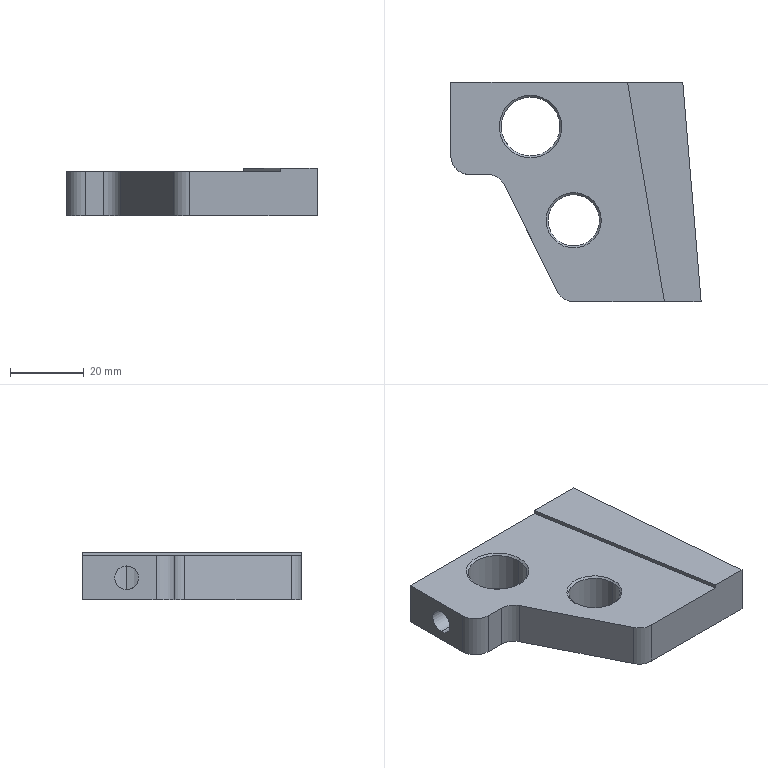Part | SolidWorks | features ICE 2, Chamfer 1, Extrusion 1 | 1 solid | 27 faces | box 68 x 59.543 x 13 mm | volume 33747 mm3 | plane 10 | cylinder 9 | cone 8 | commonest cylinder face diameters 10 x3 6.5 x2 14 x2 16 x2
STEP:
#1=CARTESIAN_POINT('',(13.645,13.,9.25));
#2=VERTEX_POINT('',#1);
#3=CARTESIAN_POINT('',(13.645,13.,2.75));
#4=VERTEX_POINT('',#3);
#5=CARTESIAN_POINT('',(13.645,13.,9.25));
#6=CARTESIAN_POINT('',(13.645,12.783,9.25));
#7=CARTESIAN_POINT('',(13.654,12.57,9.228));
#8=CARTESIAN_POINT('',(13.688,12.151,9.144));
#9=CARTESIAN_POINT('',(13.713,11.943,9.081));
#10=CARTESIAN_POINT('',(13.775,11.55,8.917));
#11=CARTESIAN_POINT('',(13.812,11.364,8.816));
#12=CARTESIAN_POINT('',(13.894,11.013,8.58));
#13=CARTESIAN_POINT('',(13.938,10.848,8.445));
#14=CARTESIAN_POINT('',(14.027,10.552,8.148));
#15=CARTESIAN_POINT('',(14.072,10.418,7.985));
#16=CARTESIAN_POINT('',(14.157,10.182,7.633));
#17=CARTESIAN_POINT('',(14.196,10.082,7.447));
#18=CARTESIAN_POINT('',(14.262,9.919,7.057));
#19=CARTESIAN_POINT('',(14.289,9.856,6.85));
#20=CARTESIAN_POINT('',(14.325,9.771,6.429));
#21=CARTESIAN_POINT('',(14.335,9.75,6.217));
#22=CARTESIAN_POINT('',(14.335,9.75,5.787));
#23=CARTESIAN_POINT('',(14.325,9.772,5.569));
#24=CARTESIAN_POINT('',(14.289,9.856,5.15));
#25=CARTESIAN_POINT('',(14.262,9.918,4.946));
#26=CARTESIAN_POINT('',(14.195,10.083,4.55));
#27=CARTESIAN_POINT('',(14.156,10.184,4.365));
#28=CARTESIAN_POINT('',(14.072,10.418,4.015));
#29=CARTESIAN_POINT('',(14.027,10.554,3.85));
#30=CARTESIAN_POINT('',(13.937,10.851,3.553));
#31=CARTESIAN_POINT('',(13.894,11.013,3.419));
#32=CARTESIAN_POINT('',(13.812,11.365,3.184));
#33=CARTESIAN_POINT('',(13.774,11.554,3.082));
#34=CARTESIAN_POINT('',(13.713,11.944,2.919));
#35=CARTESIAN_POINT('',(13.688,12.148,2.856));
#36=CARTESIAN_POINT('',(13.654,12.572,2.771));
#37=CARTESIAN_POINT('',(13.645,12.786,2.75));
#38=CARTESIAN_POINT('',(13.645,13.,2.75));
#39=B_SPLINE_CURVE_WITH_KNOTS('',3,(#5,#6,#7,#8,#9,#10,#11,#12,#13,#14,#15,#16,#17,#18,#19,#20,#21,#22,#23,#24,#25,#26,#27,#28,#29,#30,#31,#32,#33,#34,#35,#36,#37,#38),.UNSPECIFIED.,.F.,.F.,(4,2,2,2,2,2,2,2,2,2,2,2,2,2,2,2,4),(0.,0.0006421,0.001284,0.001926,0.002568,0.00321,0.003852,0.004495,0.005137,0.005779,0.006421,0.007063,0.007705,0.008347,0.008989,0.009631,0.01027),.UNSPECIFIED.);
#40=EDGE_CURVE('',#2,#4,#39,.T.);
#41=ORIENTED_EDGE('',*,*,#40,.T.);
#42=CARTESIAN_POINT('',(0.,13.,2.75));
#43=VERTEX_POINT('',#42);
#44=CARTESIAN_POINT('',(17.,13.,2.75));
#45=DIRECTION('',(-1.,0.,0.));
#46=VECTOR('',#45,1000.);
#47=LINE('',#44,#46);
#48=EDGE_CURVE('',#4,#43,#47,.T.);
#49=ORIENTED_EDGE('',*,*,#48,.T.);
#50=CARTESIAN_POINT('',(0.,13.,9.25));
#51=VERTEX_POINT('',#50);
#52=CARTESIAN_POINT('',(0.,13.,6.));
#53=DIRECTION('',(-1.,0.,0.));
#54=DIRECTION('',(0.,0.,1.));
#55=AXIS2_PLACEMENT_3D('',#52,#53,#54);
#56=CIRCLE('',#55,3.25);
#57=EDGE_CURVE('',#43,#51,#56,.T.);
#58=ORIENTED_EDGE('',*,*,#57,.T.);
#59=CARTESIAN_POINT('',(17.,13.,9.25));
#60=DIRECTION('',(-1.,0.,0.));
#61=VECTOR('',#60,1000.);
#62=LINE('',#59,#61);
#63=EDGE_CURVE('',#2,#51,#62,.T.);
#64=ORIENTED_EDGE('',*,*,#63,.F.);
#65=EDGE_LOOP('',(#41,#49,#58,#64));
#66=FACE_OUTER_BOUND('',#65,.T.);
#67=CARTESIAN_POINT('',(17.,13.,6.));
#68=DIRECTION('',(-1.,0.,0.));
#69=DIRECTION('',(0.,0.,1.));
#70=AXIS2_PLACEMENT_3D('',#67,#68,#69);
#71=CYLINDRICAL_SURFACE('',#70,3.25);
#72=ADVANCED_FACE('',(#66),#71,.F.);
#73=CARTESIAN_POINT('',(40.385,-12.47,0.5));
#74=VERTEX_POINT('',#73);
#75=CARTESIAN_POINT('',(26.385,-12.47,0.5));
#76=VERTEX_POINT('',#75);
#77=CARTESIAN_POINT('',(33.385,-12.47,0.5));
#78=DIRECTION('',(0.,0.,-1.));
#79=DIRECTION('',(1.,0.,0.));
#80=AXIS2_PLACEMENT_3D('',#77,#78,#79);
#81=CIRCLE('',#80,7.);
#82=EDGE_CURVE('',#74,#76,#81,.T.);
#83=ORIENTED_EDGE('',*,*,#82,.F.);
#84=CARTESIAN_POINT('',(40.885,-12.47,0.));
#85=VERTEX_POINT('',#84);
#86=CARTESIAN_POINT('',(40.885,-12.47,0.));
#87=DIRECTION('',(0.7071,0.,-0.7071));
#88=VECTOR('',#87,1000.);
#89=LINE('',#86,#88);
#90=EDGE_CURVE('',#74,#85,#89,.T.);
#91=ORIENTED_EDGE('',*,*,#90,.T.);
#92=CARTESIAN_POINT('',(25.885,-12.47,0.));
#93=VERTEX_POINT('',#92);
#94=CARTESIAN_POINT('',(33.385,-12.47,0.));
#95=DIRECTION('',(0.,0.,1.));
#96=DIRECTION('',(1.,0.,0.));
#97=AXIS2_PLACEMENT_3D('',#94,#95,#96);
#98=CIRCLE('',#97,7.5);
#99=EDGE_CURVE('',#93,#85,#98,.T.);
#100=ORIENTED_EDGE('',*,*,#99,.F.);
#101=CARTESIAN_POINT('',(25.885,-12.47,0.));
#102=DIRECTION('',(-0.7071,0.,-0.7071));
#103=VECTOR('',#102,1000.);
#104=LINE('',#101,#103);
#105=EDGE_CURVE('',#76,#93,#104,.T.);
#106=ORIENTED_EDGE('',*,*,#105,.F.);
#107=EDGE_LOOP('',(#83,#91,#100,#106));
#108=FACE_OUTER_BOUND('',#107,.T.);
#109=CARTESIAN_POINT('',(33.385,-12.47,0.));
#110=DIRECTION('',(0.,0.,-1.));
#111=DIRECTION('',(-1.,0.,0.));
#112=AXIS2_PLACEMENT_3D('',#109,#110,#111);
#113=CONICAL_SURFACE('',#112,7.5,0.7854);
#114=ADVANCED_FACE('',(#108),#113,.F.);
#115=CARTESIAN_POINT('',(29.645,13.,0.5));
#116=VERTEX_POINT('',#115);
#117=CARTESIAN_POINT('',(13.645,13.,0.5));
#118=VERTEX_POINT('',#117);
#119=CARTESIAN_POINT('',(21.645,13.,0.5));
#120=DIRECTION('',(0.,0.,-1.));
#121=DIRECTION('',(1.,0.,0.));
#122=AXIS2_PLACEMENT_3D('',#119,#120,#121);
#123=CIRCLE('',#122,8.);
#124=EDGE_CURVE('',#116,#118,#123,.T.);
#125=ORIENTED_EDGE('',*,*,#124,.F.);
#126=CARTESIAN_POINT('',(30.145,13.,0.));
#127=VERTEX_POINT('',#126);
#128=CARTESIAN_POINT('',(30.145,13.,0.));
#129=DIRECTION('',(0.7071,0.,-0.7071));
#130=VECTOR('',#129,1000.);
#131=LINE('',#128,#130);
#132=EDGE_CURVE('',#116,#127,#131,.T.);
#133=ORIENTED_EDGE('',*,*,#132,.T.);
#134=CARTESIAN_POINT('',(13.145,13.,0.));
#135=VERTEX_POINT('',#134);
#136=CARTESIAN_POINT('',(21.645,13.,0.));
#137=DIRECTION('',(0.,0.,1.));
#138=DIRECTION('',(1.,0.,0.));
#139=AXIS2_PLACEMENT_3D('',#136,#137,#138);
#140=CIRCLE('',#139,8.5);
#141=EDGE_CURVE('',#135,#127,#140,.T.);
#142=ORIENTED_EDGE('',*,*,#141,.F.);
#143=CARTESIAN_POINT('',(13.145,13.,0.));
#144=DIRECTION('',(-0.7071,0.,-0.7071));
#145=VECTOR('',#144,1000.);
#146=LINE('',#143,#145);
#147=EDGE_CURVE('',#118,#135,#146,.T.);
#148=ORIENTED_EDGE('',*,*,#147,.F.);
#149=EDGE_LOOP('',(#125,#133,#142,#148));
#150=FACE_OUTER_BOUND('',#149,.T.);
#151=CARTESIAN_POINT('',(21.645,13.,0.));
#152=DIRECTION('',(0.,0.,-1.));
#153=DIRECTION('',(-1.,0.,0.));
#154=AXIS2_PLACEMENT_3D('',#151,#152,#153);
#155=CONICAL_SURFACE('',#154,8.5,0.7854);
#156=ADVANCED_FACE('',(#150),#155,.F.);
#157=CARTESIAN_POINT('',(13.645,13.,11.5));
#158=VERTEX_POINT('',#157);
#159=CARTESIAN_POINT('',(29.645,13.,11.5));
#160=VERTEX_POINT('',#159);
#161=CARTESIAN_POINT('',(21.645,13.,11.5));
#162=DIRECTION('',(0.,0.,1.));
#163=DIRECTION('',(1.,0.,0.));
#164=AXIS2_PLACEMENT_3D('',#161,#162,#163);
#165=CIRCLE('',#164,8.);
#166=EDGE_CURVE('',#158,#160,#165,.T.);
#167=ORIENTED_EDGE('',*,*,#166,.F.);
#168=CARTESIAN_POINT('',(13.145,13.,12.));
#169=VERTEX_POINT('',#168);
#170=CARTESIAN_POINT('',(13.645,13.,11.5));
#171=DIRECTION('',(-0.7071,0.,0.7071));
#172=VECTOR('',#171,1000.);
#173=LINE('',#170,#172);
#174=EDGE_CURVE('',#158,#169,#173,.T.);
#175=ORIENTED_EDGE('',*,*,#174,.T.);
#176=CARTESIAN_POINT('',(30.145,13.,12.));
#177=VERTEX_POINT('',#176);
#178=CARTESIAN_POINT('',(21.645,13.,12.));
#179=DIRECTION('',(0.,0.,-1.));
#180=DIRECTION('',(1.,0.,0.));
#181=AXIS2_PLACEMENT_3D('',#178,#179,#180);
#182=CIRCLE('',#181,8.5);
#183=EDGE_CURVE('',#177,#169,#182,.T.);
#184=ORIENTED_EDGE('',*,*,#183,.F.);
#185=CARTESIAN_POINT('',(29.645,13.,11.5));
#186=DIRECTION('',(0.7071,0.,0.7071));
#187=VECTOR('',#186,1000.);
#188=LINE('',#185,#187);
#189=EDGE_CURVE('',#160,#177,#188,.T.);
#190=ORIENTED_EDGE('',*,*,#189,.F.);
#191=EDGE_LOOP('',(#167,#175,#184,#190));
#192=FACE_OUTER_BOUND('',#191,.T.);
#193=CARTESIAN_POINT('',(21.645,13.,11.5));
#194=DIRECTION('',(0.,0.,1.));
#195=DIRECTION('',(1.,0.,0.));
#196=AXIS2_PLACEMENT_3D('',#193,#194,#195);
#197=CONICAL_SURFACE('',#196,8.,0.7854);
#198=ADVANCED_FACE('',(#192),#197,.F.);
#199=CARTESIAN_POINT('',(26.385,-12.47,11.5));
#200=VERTEX_POINT('',#199);
#201=CARTESIAN_POINT('',(40.385,-12.47,11.5));
#202=VERTEX_POINT('',#201);
#203=CARTESIAN_POINT('',(33.385,-12.47,11.5));
#204=DIRECTION('',(0.,0.,1.));
#205=DIRECTION('',(1.,0.,0.));
#206=AXIS2_PLACEMENT_3D('',#203,#204,#205);
#207=CIRCLE('',#206,7.);
#208=EDGE_CURVE('',#200,#202,#207,.T.);
#209=ORIENTED_EDGE('',*,*,#208,.F.);
#210=CARTESIAN_POINT('',(25.885,-12.47,12.));
#211=VERTEX_POINT('',#210);
#212=CARTESIAN_POINT('',(26.385,-12.47,11.5));
#213=DIRECTION('',(-0.7071,0.,0.7071));
#214=VECTOR('',#213,1000.);
#215=LINE('',#212,#214);
#216=EDGE_CURVE('',#200,#211,#215,.T.);
#217=ORIENTED_EDGE('',*,*,#216,.T.);
#218=CARTESIAN_POINT('',(40.885,-12.47,12.));
#219=VERTEX_POINT('',#218);
#220=CARTESIAN_POINT('',(33.385,-12.47,12.));
#221=DIRECTION('',(0.,0.,-1.));
#222=DIRECTION('',(1.,0.,0.));
#223=AXIS2_PLACEMENT_3D('',#220,#221,#222);
#224=CIRCLE('',#223,7.5);
#225=EDGE_CURVE('',#219,#211,#224,.T.);
#226=ORIENTED_EDGE('',*,*,#225,.F.);
#227=CARTESIAN_POINT('',(40.385,-12.47,11.5));
#228=DIRECTION('',(0.7071,0.,0.7071));
#229=VECTOR('',#228,1000.);
#230=LINE('',#227,#229);
#231=EDGE_CURVE('',#202,#219,#230,.T.);
#232=ORIENTED_EDGE('',*,*,#231,.F.);
#233=EDGE_LOOP('',(#209,#217,#226,#232));
#234=FACE_OUTER_BOUND('',#233,.T.);
#235=CARTESIAN_POINT('',(33.385,-12.47,11.5));
#236=DIRECTION('',(0.,0.,1.));
#237=DIRECTION('',(1.,0.,0.));
#238=AXIS2_PLACEMENT_3D('',#235,#236,#237);
#239=CONICAL_SURFACE('',#238,7.,0.7854);
#240=ADVANCED_FACE('',(#234),#239,.F.);
#241=ORIENTED_EDGE('',*,*,#208,.T.);
#242=CARTESIAN_POINT('',(40.385,-12.47,13.));
#243=DIRECTION('',(0.,0.,-1.));
#244=VECTOR('',#243,1000.);
#245=LINE('',#242,#244);
#246=EDGE_CURVE('',#202,#74,#245,.T.);
#247=ORIENTED_EDGE('',*,*,#246,.T.);
#248=ORIENTED_EDGE('',*,*,#82,.T.);
#249=CARTESIAN_POINT('',(26.385,-12.47,13.));
#250=DIRECTION('',(0.,0.,-1.));
#251=VECTOR('',#250,1000.);
#252=LINE('',#249,#251);
#253=EDGE_CURVE('',#200,#76,#252,.T.);
#254=ORIENTED_EDGE('',*,*,#253,.F.);
#255=EDGE_LOOP('',(#241,#247,#248,#254));
#256=FACE_OUTER_BOUND('',#255,.T.);
#257=CARTESIAN_POINT('',(33.385,-12.47,13.));
#258=DIRECTION('',(0.,0.,-1.));
#259=DIRECTION('',(-1.,0.,0.));
#260=AXIS2_PLACEMENT_3D('',#257,#258,#259);
#261=CYLINDRICAL_SURFACE('',#260,7.);
#262=ADVANCED_FACE('',(#256),#261,.F.);
#263=ORIENTED_EDGE('',*,*,#166,.T.);
#264=CARTESIAN_POINT('',(29.645,13.,13.));
#265=DIRECTION('',(0.,0.,-1.));
#266=VECTOR('',#265,1000.);
#267=LINE('',#264,#266);
#268=EDGE_CURVE('',#160,#116,#267,.T.);
#269=ORIENTED_EDGE('',*,*,#268,.T.);
#270=ORIENTED_EDGE('',*,*,#124,.T.);
#271=CARTESIAN_POINT('',(13.645,13.,13.));
#272=DIRECTION('',(0.,0.,-1.));
#273=VECTOR('',#272,1000.);
#274=LINE('',#271,#273);
#275=EDGE_CURVE('',#4,#118,#274,.T.);
#276=ORIENTED_EDGE('',*,*,#275,.F.);
#277=ORIENTED_EDGE('',*,*,#40,.F.);
#278=CARTESIAN_POINT('',(13.645,13.,13.));
#279=DIRECTION('',(0.,0.,-1.));
#280=VECTOR('',#279,1000.);
#281=LINE('',#278,#280);
#282=EDGE_CURVE('',#158,#2,#281,.T.);
#283=ORIENTED_EDGE('',*,*,#282,.F.);
#284=EDGE_LOOP('',(#263,#269,#270,#276,#277,#283));
#285=FACE_OUTER_BOUND('',#284,.T.);
#286=CARTESIAN_POINT('',(21.645,13.,13.));
#287=DIRECTION('',(0.,0.,-1.));
#288=DIRECTION('',(-1.,0.,0.));
#289=AXIS2_PLACEMENT_3D('',#286,#287,#288);
#290=CYLINDRICAL_SURFACE('',#289,8.);
#291=ADVANCED_FACE('',(#285),#290,.F.);
#292=CARTESIAN_POINT('',(0.,13.,6.));
#293=DIRECTION('',(-1.,0.,0.));
#294=DIRECTION('',(0.,0.,1.));
#295=AXIS2_PLACEMENT_3D('',#292,#293,#294);
#296=CIRCLE('',#295,3.25);
#297=EDGE_CURVE('',#51,#43,#296,.T.);
#298=ORIENTED_EDGE('',*,*,#297,.F.);
#299=ORIENTED_EDGE('',*,*,#57,.F.);
#300=EDGE_LOOP('',(#298,#299));
#301=FACE_BOUND('',#300,.T.);
#302=CARTESIAN_POINT('',(0.,25.,12.));
#303=VERTEX_POINT('',#302);
#304=CARTESIAN_POINT('',(0.,5.,12.));
#305=VERTEX_POINT('',#304);
#306=CARTESIAN_POINT('',(0.,25.,12.));
#307=DIRECTION('',(0.,-1.,0.));
#308=VECTOR('',#307,1000.);
#309=LINE('',#306,#308);
#310=EDGE_CURVE('',#303,#305,#309,.T.);
#311=ORIENTED_EDGE('',*,*,#310,.F.);
#312=CARTESIAN_POINT('',(0.,25.,0.));
#313=VERTEX_POINT('',#312);
#314=CARTESIAN_POINT('',(0.,25.,13.));
#315=DIRECTION('',(0.,0.,-1.));
#316=VECTOR('',#315,1000.);
#317=LINE('',#314,#316);
#318=EDGE_CURVE('',#303,#313,#317,.T.);
#319=ORIENTED_EDGE('',*,*,#318,.T.);
#320=CARTESIAN_POINT('',(0.,5.,0.));
#321=VERTEX_POINT('',#320);
#322=CARTESIAN_POINT('',(0.,5.,0.));
#323=DIRECTION('',(0.,-1.,0.));
#324=VECTOR('',#323,1000.);
#325=LINE('',#322,#324);
#326=EDGE_CURVE('',#313,#321,#325,.T.);
#327=ORIENTED_EDGE('',*,*,#326,.T.);
#328=CARTESIAN_POINT('',(0.,5.,13.));
#329=DIRECTION('',(0.,0.,-1.));
#330=VECTOR('',#329,1000.);
#331=LINE('',#328,#330);
#332=EDGE_CURVE('',#305,#321,#331,.T.);
#333=ORIENTED_EDGE('',*,*,#332,.F.);
#334=EDGE_LOOP('',(#311,#319,#327,#333));
#335=FACE_OUTER_BOUND('',#334,.T.);
#336=CARTESIAN_POINT('',(0.,5.,13.));
#337=DIRECTION('',(1.,0.,0.));
#338=DIRECTION('',(0.,0.,-1.));
#339=AXIS2_PLACEMENT_3D('',#336,#337,#338);
#340=PLANE('',#339);
#341=ADVANCED_FACE('',(#301,#335),#340,.F.);
#342=CARTESIAN_POINT('',(5.,0.,12.));
#343=VERTEX_POINT('',#342);
#344=CARTESIAN_POINT('',(5.,5.,12.));
#345=DIRECTION('',(0.,0.,1.));
#346=DIRECTION('',(1.,0.,0.));
#347=AXIS2_PLACEMENT_3D('',#344,#345,#346);
#348=CIRCLE('',#347,5.);
#349=EDGE_CURVE('',#305,#343,#348,.T.);
#350=ORIENTED_EDGE('',*,*,#349,.F.);
#351=ORIENTED_EDGE('',*,*,#332,.T.);
#352=CARTESIAN_POINT('',(5.,0.,0.));
#353=VERTEX_POINT('',#352);
#354=CARTESIAN_POINT('',(5.,5.,0.));
#355=DIRECTION('',(0.,0.,1.));
#356=DIRECTION('',(-1.,0.,0.));
#357=AXIS2_PLACEMENT_3D('',#354,#355,#356);
#358=CIRCLE('',#357,5.);
#359=EDGE_CURVE('',#321,#353,#358,.T.);
#360=ORIENTED_EDGE('',*,*,#359,.T.);
#361=CARTESIAN_POINT('',(5.,0.,13.));
#362=DIRECTION('',(0.,0.,-1.));
#363=VECTOR('',#362,1000.);
#364=LINE('',#361,#363);
#365=EDGE_CURVE('',#343,#353,#364,.T.);
#366=ORIENTED_EDGE('',*,*,#365,.F.);
#367=EDGE_LOOP('',(#350,#351,#360,#366));
#368=FACE_OUTER_BOUND('',#367,.T.);
#369=CARTESIAN_POINT('',(5.,5.,13.));
#370=DIRECTION('',(0.,0.,-1.));
#371=DIRECTION('',(-1.,0.,0.));
#372=AXIS2_PLACEMENT_3D('',#369,#370,#371);
#373=CYLINDRICAL_SURFACE('',#372,5.);
#374=ADVANCED_FACE('',(#368),#373,.T.);
#375=CARTESIAN_POINT('',(9.997,0.,12.));
#376=VERTEX_POINT('',#375);
#377=CARTESIAN_POINT('',(5.,0.,12.));
#378=DIRECTION('',(1.,0.,0.));
#379=VECTOR('',#378,1000.);
#380=LINE('',#377,#379);
#381=EDGE_CURVE('',#343,#376,#380,.T.);
#382=ORIENTED_EDGE('',*,*,#381,.F.);
#383=ORIENTED_EDGE('',*,*,#365,.T.);
#384=CARTESIAN_POINT('',(9.997,0.,0.));
#385=VERTEX_POINT('',#384);
#386=CARTESIAN_POINT('',(9.997,0.,0.));
#387=DIRECTION('',(1.,0.,0.));
#388=VECTOR('',#387,1000.);
#389=LINE('',#386,#388);
#390=EDGE_CURVE('',#353,#385,#389,.T.);
#391=ORIENTED_EDGE('',*,*,#390,.T.);
#392=CARTESIAN_POINT('',(9.997,0.,13.));
#393=DIRECTION('',(0.,0.,-1.));
#394=VECTOR('',#393,1000.);
#395=LINE('',#392,#394);
#396=EDGE_CURVE('',#376,#385,#395,.T.);
#397=ORIENTED_EDGE('',*,*,#396,.F.);
#398=EDGE_LOOP('',(#382,#383,#391,#397));
#399=FACE_OUTER_BOUND('',#398,.T.);
#400=CARTESIAN_POINT('',(9.997,0.,13.));
#401=DIRECTION('',(0.,1.,0.));
#402=DIRECTION('',(0.,0.,1.));
#403=AXIS2_PLACEMENT_3D('',#400,#401,#402);
#404=PLANE('',#403);
#405=ADVANCED_FACE('',(#399),#404,.F.);
#406=CARTESIAN_POINT('',(14.473,-2.772,12.));
#407=VERTEX_POINT('',#406);
#408=CARTESIAN_POINT('',(9.997,-5.,12.));
#409=DIRECTION('',(0.,0.,-1.));
#410=DIRECTION('',(1.,0.,0.));
#411=AXIS2_PLACEMENT_3D('',#408,#409,#410);
#412=CIRCLE('',#411,5.);
#413=EDGE_CURVE('',#376,#407,#412,.T.);
#414=ORIENTED_EDGE('',*,*,#413,.F.);
#415=ORIENTED_EDGE('',*,*,#396,.T.);
#416=CARTESIAN_POINT('',(14.473,-2.772,0.));
#417=VERTEX_POINT('',#416);
#418=CARTESIAN_POINT('',(9.997,-5.,0.));
#419=DIRECTION('',(0.,0.,-1.));
#420=DIRECTION('',(-1.,0.,0.));
#421=AXIS2_PLACEMENT_3D('',#418,#419,#420);
#422=CIRCLE('',#421,5.);
#423=EDGE_CURVE('',#385,#417,#422,.T.);
#424=ORIENTED_EDGE('',*,*,#423,.T.);
#425=CARTESIAN_POINT('',(14.473,-2.772,13.));
#426=DIRECTION('',(0.,0.,-1.));
#427=VECTOR('',#426,1000.);
#428=LINE('',#425,#427);
#429=EDGE_CURVE('',#407,#417,#428,.T.);
#430=ORIENTED_EDGE('',*,*,#429,.F.);
#431=EDGE_LOOP('',(#414,#415,#424,#430));
#432=FACE_OUTER_BOUND('',#431,.T.);
#433=CARTESIAN_POINT('',(9.997,-5.,13.));
#434=DIRECTION('',(0.,0.,-1.));
#435=DIRECTION('',(-1.,0.,0.));
#436=AXIS2_PLACEMENT_3D('',#433,#434,#435);
#437=CYLINDRICAL_SURFACE('',#436,5.);
#438=ADVANCED_FACE('',(#432),#437,.F.);
#439=CARTESIAN_POINT('',(28.909,-31.772,12.));
#440=VERTEX_POINT('',#439);
#441=CARTESIAN_POINT('',(14.473,-2.772,12.));
#442=DIRECTION('',(0.4456,-0.8952,0.));
#443=VECTOR('',#442,1000.);
#444=LINE('',#441,#443);
#445=EDGE_CURVE('',#407,#440,#444,.T.);
#446=ORIENTED_EDGE('',*,*,#445,.F.);
#447=ORIENTED_EDGE('',*,*,#429,.T.);
#448=CARTESIAN_POINT('',(28.909,-31.772,0.));
#449=VERTEX_POINT('',#448);
#450=CARTESIAN_POINT('',(28.909,-31.772,0.));
#451=DIRECTION('',(0.4456,-0.8952,0.));
#452=VECTOR('',#451,1000.);
#453=LINE('',#450,#452);
#454=EDGE_CURVE('',#417,#449,#453,.T.);
#455=ORIENTED_EDGE('',*,*,#454,.T.);
#456=CARTESIAN_POINT('',(28.909,-31.772,13.));
#457=DIRECTION('',(0.,0.,-1.));
#458=VECTOR('',#457,1000.);
#459=LINE('',#456,#458);
#460=EDGE_CURVE('',#440,#449,#459,.T.);
#461=ORIENTED_EDGE('',*,*,#460,.F.);
#462=EDGE_LOOP('',(#446,#447,#455,#461));
#463=FACE_OUTER_BOUND('',#462,.T.);
#464=CARTESIAN_POINT('',(28.909,-31.772,13.));
#465=DIRECTION('',(0.8952,0.4456,0.));
#466=DIRECTION('',(-0.4456,0.8952,0.));
#467=AXIS2_PLACEMENT_3D('',#464,#465,#466);
#468=PLANE('',#467);
#469=ADVANCED_FACE('',(#463),#468,.F.);
#470=CARTESIAN_POINT('',(33.385,-34.543,12.));
#471=VERTEX_POINT('',#470);
#472=CARTESIAN_POINT('',(33.385,-29.543,12.));
#473=DIRECTION('',(0.,0.,1.));
#474=DIRECTION('',(1.,0.,0.));
#475=AXIS2_PLACEMENT_3D('',#472,#473,#474);
#476=CIRCLE('',#475,5.);
#477=EDGE_CURVE('',#440,#471,#476,.T.);
#478=ORIENTED_EDGE('',*,*,#477,.F.);
#479=ORIENTED_EDGE('',*,*,#460,.T.);
#480=CARTESIAN_POINT('',(33.385,-34.543,0.));
#481=VERTEX_POINT('',#480);
#482=CARTESIAN_POINT('',(33.385,-29.543,0.));
#483=DIRECTION('',(0.,0.,1.));
#484=DIRECTION('',(1.,0.,0.));
#485=AXIS2_PLACEMENT_3D('',#482,#483,#484);
#486=CIRCLE('',#485,5.);
#487=EDGE_CURVE('',#449,#481,#486,.T.);
#488=ORIENTED_EDGE('',*,*,#487,.T.);
#489=CARTESIAN_POINT('',(33.385,-34.543,13.));
#490=DIRECTION('',(0.,0.,-1.));
#491=VECTOR('',#490,1000.);
#492=LINE('',#489,#491);
#493=EDGE_CURVE('',#471,#481,#492,.T.);
#494=ORIENTED_EDGE('',*,*,#493,.F.);
#495=EDGE_LOOP('',(#478,#479,#488,#494));
#496=FACE_OUTER_BOUND('',#495,.T.);
#497=CARTESIAN_POINT('',(33.385,-29.543,13.));
#498=DIRECTION('',(0.,0.,-1.));
#499=DIRECTION('',(-1.,0.,0.));
#500=AXIS2_PLACEMENT_3D('',#497,#498,#499);
#501=CYLINDRICAL_SURFACE('',#500,5.);
#502=ADVANCED_FACE('',(#496),#501,.T.);
#503=ORIENTED_EDGE('',*,*,#268,.F.);
#504=CARTESIAN_POINT('',(21.645,13.,11.5));
#505=DIRECTION('',(0.,0.,1.));
#506=DIRECTION('',(1.,0.,0.));
#507=AXIS2_PLACEMENT_3D('',#504,#505,#506);
#508=CIRCLE('',#507,8.);
#509=EDGE_CURVE('',#160,#158,#508,.T.);
#510=ORIENTED_EDGE('',*,*,#509,.T.);
#511=ORIENTED_EDGE('',*,*,#282,.T.);
#512=CARTESIAN_POINT('',(13.645,13.,2.75));
#513=CARTESIAN_POINT('',(13.645,13.214,2.75));
#514=CARTESIAN_POINT('',(13.654,13.431,2.772));
#515=CARTESIAN_POINT('',(13.688,13.852,2.856));
#516=CARTESIAN_POINT('',(13.713,14.055,2.919));
#517=CARTESIAN_POINT('',(13.775,14.449,3.083));
#518=CARTESIAN_POINT('',(13.812,14.638,3.185));
#519=CARTESIAN_POINT('',(13.894,14.987,3.42));
#520=CARTESIAN_POINT('',(13.938,15.15,3.554));
#521=CARTESIAN_POINT('',(14.028,15.45,3.854));
#522=CARTESIAN_POINT('',(14.072,15.582,4.016));
#523=CARTESIAN_POINT('',(14.156,15.816,4.365));
#524=CARTESIAN_POINT('',(14.196,15.918,4.554));
#525=CARTESIAN_POINT('',(14.262,16.082,4.946));
#526=CARTESIAN_POINT('',(14.289,16.144,5.148));
#527=CARTESIAN_POINT('',(14.325,16.228,5.567));
#528=CARTESIAN_POINT('',(14.335,16.25,5.785));
#529=CARTESIAN_POINT('',(14.335,16.25,6.214));
#530=CARTESIAN_POINT('',(14.326,16.229,6.427));
#531=CARTESIAN_POINT('',(14.289,16.144,6.85));
#532=CARTESIAN_POINT('',(14.262,16.081,7.055));
#533=CARTESIAN_POINT('',(14.196,15.918,7.446));
#534=CARTESIAN_POINT('',(14.156,15.816,7.635));
#535=CARTESIAN_POINT('',(14.072,15.581,7.986));
#536=CARTESIAN_POINT('',(14.027,15.448,8.148));
#537=CARTESIAN_POINT('',(13.938,15.15,8.446));
#538=CARTESIAN_POINT('',(13.893,14.986,8.582));
#539=CARTESIAN_POINT('',(13.812,14.637,8.816));
#540=CARTESIAN_POINT('',(13.775,14.451,8.916));
#541=CARTESIAN_POINT('',(13.712,14.055,9.082));
#542=CARTESIAN_POINT('',(13.688,13.851,9.144));
#543=CARTESIAN_POINT('',(13.654,13.433,9.228));
#544=CARTESIAN_POINT('',(13.645,13.217,9.25));
#545=CARTESIAN_POINT('',(13.645,13.,9.25));
#546=B_SPLINE_CURVE_WITH_KNOTS('',3,(#512,#513,#514,#515,#516,#517,#518,#519,#520,#521,#522,#523,#524,#525,#526,#527,#528,#529,#530,#531,#532,#533,#534,#535,#536,#537,#538,#539,#540,#541,#542,#543,#544,#545),.UNSPECIFIED.,.F.,.F.,(4,2,2,2,2,2,2,2,2,2,2,2,2,2,2,2,4),(0.01027,0.01091,0.01156,0.0122,0.01284,0.01348,0.01412,0.01476,0.01541,0.01605,0.01669,0.01733,0.01797,0.01861,0.01926,0.0199,0.02054),.UNSPECIFIED.);
#547=EDGE_CURVE('',#4,#2,#546,.T.);
#548=ORIENTED_EDGE('',*,*,#547,.F.);
#549=ORIENTED_EDGE('',*,*,#275,.T.);
#550=CARTESIAN_POINT('',(21.645,13.,0.5));
#551=DIRECTION('',(0.,0.,-1.));
#552=DIRECTION('',(1.,0.,0.));
#553=AXIS2_PLACEMENT_3D('',#550,#551,#552);
#554=CIRCLE('',#553,8.);
#555=EDGE_CURVE('',#118,#116,#554,.T.);
#556=ORIENTED_EDGE('',*,*,#555,.T.);
#557=EDGE_LOOP('',(#503,#510,#511,#548,#549,#556));
#558=FACE_OUTER_BOUND('',#557,.T.);
#559=CARTESIAN_POINT('',(21.645,13.,13.));
#560=DIRECTION('',(0.,0.,-1.));
#561=DIRECTION('',(-1.,0.,0.));
#562=AXIS2_PLACEMENT_3D('',#559,#560,#561);
#563=CYLINDRICAL_SURFACE('',#562,8.);
#564=ADVANCED_FACE('',(#558),#563,.F.);
#565=ORIENTED_EDGE('',*,*,#246,.F.);
#566=CARTESIAN_POINT('',(33.385,-12.47,11.5));
#567=DIRECTION('',(0.,0.,1.));
#568=DIRECTION('',(1.,0.,0.));
#569=AXIS2_PLACEMENT_3D('',#566,#567,#568);
#570=CIRCLE('',#569,7.);
#571=EDGE_CURVE('',#202,#200,#570,.T.);
#572=ORIENTED_EDGE('',*,*,#571,.T.);
#573=ORIENTED_EDGE('',*,*,#253,.T.);
#574=CARTESIAN_POINT('',(33.385,-12.47,0.5));
#575=DIRECTION('',(0.,0.,-1.));
#576=DIRECTION('',(1.,0.,0.));
#577=AXIS2_PLACEMENT_3D('',#574,#575,#576);
#578=CIRCLE('',#577,7.);
#579=EDGE_CURVE('',#76,#74,#578,.T.);
#580=ORIENTED_EDGE('',*,*,#579,.T.);
#581=EDGE_LOOP('',(#565,#572,#573,#580));
#582=FACE_OUTER_BOUND('',#581,.T.);
#583=CARTESIAN_POINT('',(33.385,-12.47,13.));
#584=DIRECTION('',(0.,0.,-1.));
#585=DIRECTION('',(-1.,0.,0.));
#586=AXIS2_PLACEMENT_3D('',#583,#584,#585);
#587=CYLINDRICAL_SURFACE('',#586,7.);
#588=ADVANCED_FACE('',(#582),#587,.F.);
#589=CARTESIAN_POINT('',(58.,-34.543,13.));
#590=VERTEX_POINT('',#589);
#591=CARTESIAN_POINT('',(48.,25.,13.));
#592=VERTEX_POINT('',#591);
#593=CARTESIAN_POINT('',(48.,25.,13.));
#594=DIRECTION('',(-0.1656,0.9862,0.));
#595=VECTOR('',#594,1000.);
#596=LINE('',#593,#595);
#597=EDGE_CURVE('',#590,#592,#596,.T.);
#598=ORIENTED_EDGE('',*,*,#597,.F.);
#599=CARTESIAN_POINT('',(68.,-34.543,13.));
#600=VERTEX_POINT('',#599);
#601=CARTESIAN_POINT('',(68.,-34.543,13.));
#602=DIRECTION('',(1.,0.,0.));
#603=VECTOR('',#602,1000.);
#604=LINE('',#601,#603);
#605=EDGE_CURVE('',#590,#600,#604,.T.);
#606=ORIENTED_EDGE('',*,*,#605,.T.);
#607=CARTESIAN_POINT('',(63.,25.,13.));
#608=VERTEX_POINT('',#607);
#609=CARTESIAN_POINT('',(63.,25.,13.));
#610=DIRECTION('',(-0.08368,0.9965,0.));
#611=VECTOR('',#610,1000.);
#612=LINE('',#609,#611);
#613=EDGE_CURVE('',#600,#608,#612,.T.);
#614=ORIENTED_EDGE('',*,*,#613,.T.);
#615=CARTESIAN_POINT('',(0.,25.,13.));
#616=DIRECTION('',(-1.,0.,0.));
#617=VECTOR('',#616,1000.);
#618=LINE('',#615,#617);
#619=EDGE_CURVE('',#608,#592,#618,.T.);
#620=ORIENTED_EDGE('',*,*,#619,.T.);
#621=EDGE_LOOP('',(#598,#606,#614,#620));
#622=FACE_OUTER_BOUND('',#621,.T.);
#623=CARTESIAN_POINT('',(33.385,-29.543,13.));
#624=DIRECTION('',(0.,0.,1.));
#625=DIRECTION('',(1.,0.,0.));
#626=AXIS2_PLACEMENT_3D('',#623,#624,#625);
#627=PLANE('',#626);
#628=ADVANCED_FACE('',(#622),#627,.T.);
#629=ORIENTED_EDGE('',*,*,#141,.T.);
#630=CARTESIAN_POINT('',(21.645,13.,0.));
#631=DIRECTION('',(0.,0.,1.));
#632=DIRECTION('',(1.,0.,0.));
#633=AXIS2_PLACEMENT_3D('',#630,#631,#632);
#634=CIRCLE('',#633,8.5);
#635=EDGE_CURVE('',#127,#135,#634,.T.);
#636=ORIENTED_EDGE('',*,*,#635,.T.);
#637=EDGE_LOOP('',(#629,#636));
#638=FACE_BOUND('',#637,.T.);
#639=ORIENTED_EDGE('',*,*,#99,.T.);
#640=CARTESIAN_POINT('',(33.385,-12.47,0.));
#641=DIRECTION('',(0.,0.,1.));
#642=DIRECTION('',(1.,0.,0.));
#643=AXIS2_PLACEMENT_3D('',#640,#641,#642);
#644=CIRCLE('',#643,7.5);
#645=EDGE_CURVE('',#85,#93,#644,.T.);
#646=ORIENTED_EDGE('',*,*,#645,.T.);
#647=EDGE_LOOP('',(#639,#646));
#648=FACE_BOUND('',#647,.T.);
#649=CARTESIAN_POINT('',(63.,25.,0.));
#650=VERTEX_POINT('',#649);
#651=CARTESIAN_POINT('',(0.,25.,0.));
#652=DIRECTION('',(-1.,0.,0.));
#653=VECTOR('',#652,1000.);
#654=LINE('',#651,#653);
#655=EDGE_CURVE('',#650,#313,#654,.T.);
#656=ORIENTED_EDGE('',*,*,#655,.F.);
#657=CARTESIAN_POINT('',(68.,-34.543,0.));
#658=VERTEX_POINT('',#657);
#659=CARTESIAN_POINT('',(63.,25.,0.));
#660=DIRECTION('',(-0.08368,0.9965,0.));
#661=VECTOR('',#660,1000.);
#662=LINE('',#659,#661);
#663=EDGE_CURVE('',#658,#650,#662,.T.);
#664=ORIENTED_EDGE('',*,*,#663,.F.);
#665=CARTESIAN_POINT('',(68.,-34.543,0.));
#666=DIRECTION('',(1.,0.,0.));
#667=VECTOR('',#666,1000.);
#668=LINE('',#665,#667);
#669=EDGE_CURVE('',#481,#658,#668,.T.);
#670=ORIENTED_EDGE('',*,*,#669,.F.);
#671=ORIENTED_EDGE('',*,*,#487,.F.);
#672=ORIENTED_EDGE('',*,*,#454,.F.);
#673=ORIENTED_EDGE('',*,*,#423,.F.);
#674=ORIENTED_EDGE('',*,*,#390,.F.);
#675=ORIENTED_EDGE('',*,*,#359,.F.);
#676=ORIENTED_EDGE('',*,*,#326,.F.);
#677=EDGE_LOOP('',(#656,#664,#670,#671,#672,#673,#674,#675,#676));
#678=FACE_OUTER_BOUND('',#677,.T.);
#679=CARTESIAN_POINT('',(33.385,-29.543,0.));
#680=DIRECTION('',(0.,0.,1.));
#681=DIRECTION('',(1.,0.,0.));
#682=AXIS2_PLACEMENT_3D('',#679,#680,#681);
#683=PLANE('',#682);
#684=ADVANCED_FACE('',(#638,#648,#678),#683,.F.);
#685=CARTESIAN_POINT('',(48.,25.,12.));
#686=VERTEX_POINT('',#685);
#687=CARTESIAN_POINT('',(48.,25.,12.));
#688=DIRECTION('',(-1.,0.,0.));
#689=VECTOR('',#688,1000.);
#690=LINE('',#687,#689);
#691=EDGE_CURVE('',#686,#303,#690,.T.);
#692=ORIENTED_EDGE('',*,*,#691,.F.);
#693=CARTESIAN_POINT('',(48.,25.,12.));
#694=DIRECTION('',(0.,0.,1.));
#695=VECTOR('',#694,1000.);
#696=LINE('',#693,#695);
#697=EDGE_CURVE('',#686,#592,#696,.T.);
#698=ORIENTED_EDGE('',*,*,#697,.T.);
#699=ORIENTED_EDGE('',*,*,#619,.F.);
#700=CARTESIAN_POINT('',(63.,25.,13.));
#701=DIRECTION('',(0.,0.,-1.));
#702=VECTOR('',#701,1000.);
#703=LINE('',#700,#702);
#704=EDGE_CURVE('',#608,#650,#703,.T.);
#705=ORIENTED_EDGE('',*,*,#704,.T.);
#706=ORIENTED_EDGE('',*,*,#655,.T.);
#707=ORIENTED_EDGE('',*,*,#318,.F.);
#708=EDGE_LOOP('',(#692,#698,#699,#705,#706,#707));
#709=FACE_OUTER_BOUND('',#708,.T.);
#710=CARTESIAN_POINT('',(0.,25.,13.));
#711=DIRECTION('',(0.,-1.,0.));
#712=DIRECTION('',(0.,0.,-1.));
#713=AXIS2_PLACEMENT_3D('',#710,#711,#712);
#714=PLANE('',#713);
#715=ADVANCED_FACE('',(#709),#714,.F.);
#716=ORIENTED_EDGE('',*,*,#605,.F.);
#717=CARTESIAN_POINT('',(58.,-34.543,12.));
#718=VERTEX_POINT('',#717);
#719=CARTESIAN_POINT('',(58.,-34.543,12.));
#720=DIRECTION('',(0.,0.,1.));
#721=VECTOR('',#720,1000.);
#722=LINE('',#719,#721);
#723=EDGE_CURVE('',#718,#590,#722,.T.);
#724=ORIENTED_EDGE('',*,*,#723,.F.);
#725=CARTESIAN_POINT('',(33.385,-34.543,12.));
#726=DIRECTION('',(1.,0.,0.));
#727=VECTOR('',#726,1000.);
#728=LINE('',#725,#727);
#729=EDGE_CURVE('',#471,#718,#728,.T.);
#730=ORIENTED_EDGE('',*,*,#729,.F.);
#731=ORIENTED_EDGE('',*,*,#493,.T.);
#732=ORIENTED_EDGE('',*,*,#669,.T.);
#733=CARTESIAN_POINT('',(68.,-34.543,13.));
#734=DIRECTION('',(0.,0.,-1.));
#735=VECTOR('',#734,1000.);
#736=LINE('',#733,#735);
#737=EDGE_CURVE('',#600,#658,#736,.T.);
#738=ORIENTED_EDGE('',*,*,#737,.F.);
#739=EDGE_LOOP('',(#716,#724,#730,#731,#732,#738));
#740=FACE_OUTER_BOUND('',#739,.T.);
#741=CARTESIAN_POINT('',(68.,-34.543,13.));
#742=DIRECTION('',(0.,1.,0.));
#743=DIRECTION('',(0.,0.,1.));
#744=AXIS2_PLACEMENT_3D('',#741,#742,#743);
#745=PLANE('',#744);
#746=ADVANCED_FACE('',(#740),#745,.F.);
#747=ORIENTED_EDGE('',*,*,#663,.T.);
#748=ORIENTED_EDGE('',*,*,#704,.F.);
#749=ORIENTED_EDGE('',*,*,#613,.F.);
#750=ORIENTED_EDGE('',*,*,#737,.T.);
#751=EDGE_LOOP('',(#747,#748,#749,#750));
#752=FACE_OUTER_BOUND('',#751,.T.);
#753=CARTESIAN_POINT('',(63.,25.,13.));
#754=DIRECTION('',(-0.9965,-0.08368,0.));
#755=DIRECTION('',(0.08368,-0.9965,0.));
#756=AXIS2_PLACEMENT_3D('',#753,#754,#755);
#757=PLANE('',#756);
#758=ADVANCED_FACE('',(#752),#757,.F.);
#759=ORIENTED_EDGE('',*,*,#597,.T.);
#760=ORIENTED_EDGE('',*,*,#697,.F.);
#761=CARTESIAN_POINT('',(48.,25.,12.));
#762=DIRECTION('',(-0.1656,0.9862,0.));
#763=VECTOR('',#762,1000.);
#764=LINE('',#761,#763);
#765=EDGE_CURVE('',#718,#686,#764,.T.);
#766=ORIENTED_EDGE('',*,*,#765,.F.);
#767=ORIENTED_EDGE('',*,*,#723,.T.);
#768=EDGE_LOOP('',(#759,#760,#766,#767));
#769=FACE_OUTER_BOUND('',#768,.T.);
#770=CARTESIAN_POINT('',(48.,25.,12.));
#771=DIRECTION('',(0.9862,0.1656,0.));
#772=DIRECTION('',(-0.1656,0.9862,0.));
#773=AXIS2_PLACEMENT_3D('',#770,#771,#772);
#774=PLANE('',#773);
#775=ADVANCED_FACE('',(#769),#774,.F.);
#776=ORIENTED_EDGE('',*,*,#225,.T.);
#777=CARTESIAN_POINT('',(33.385,-12.47,12.));
#778=DIRECTION('',(0.,0.,-1.));
#779=DIRECTION('',(1.,0.,0.));
#780=AXIS2_PLACEMENT_3D('',#777,#778,#779);
#781=CIRCLE('',#780,7.5);
#782=EDGE_CURVE('',#211,#219,#781,.T.);
#783=ORIENTED_EDGE('',*,*,#782,.T.);
#784=EDGE_LOOP('',(#776,#783));
#785=FACE_BOUND('',#784,.T.);
#786=ORIENTED_EDGE('',*,*,#183,.T.);
#787=CARTESIAN_POINT('',(21.645,13.,12.));
#788=DIRECTION('',(0.,0.,-1.));
#789=DIRECTION('',(1.,0.,0.));
#790=AXIS2_PLACEMENT_3D('',#787,#788,#789);
#791=CIRCLE('',#790,8.5);
#792=EDGE_CURVE('',#169,#177,#791,.T.);
#793=ORIENTED_EDGE('',*,*,#792,.T.);
#794=EDGE_LOOP('',(#786,#793));
#795=FACE_BOUND('',#794,.T.);
#796=ORIENTED_EDGE('',*,*,#310,.T.);
#797=ORIENTED_EDGE('',*,*,#349,.T.);
#798=ORIENTED_EDGE('',*,*,#381,.T.);
#799=ORIENTED_EDGE('',*,*,#413,.T.);
#800=ORIENTED_EDGE('',*,*,#445,.T.);
#801=ORIENTED_EDGE('',*,*,#477,.T.);
#802=ORIENTED_EDGE('',*,*,#729,.T.);
#803=ORIENTED_EDGE('',*,*,#765,.T.);
#804=ORIENTED_EDGE('',*,*,#691,.T.);
#805=EDGE_LOOP('',(#796,#797,#798,#799,#800,#801,#802,#803,#804));
#806=FACE_OUTER_BOUND('',#805,.T.);
#807=CARTESIAN_POINT('',(5.,5.,12.));
#808=DIRECTION('',(0.,0.,1.));
#809=DIRECTION('',(1.,0.,0.));
#810=AXIS2_PLACEMENT_3D('',#807,#808,#809);
#811=PLANE('',#810);
#812=ADVANCED_FACE('',(#785,#795,#806),#811,.T.);
#813=ORIENTED_EDGE('',*,*,#216,.F.);
#814=ORIENTED_EDGE('',*,*,#571,.F.);
#815=ORIENTED_EDGE('',*,*,#231,.T.);
#816=ORIENTED_EDGE('',*,*,#782,.F.);
#817=EDGE_LOOP('',(#813,#814,#815,#816));
#818=FACE_OUTER_BOUND('',#817,.T.);
#819=CARTESIAN_POINT('',(33.385,-12.47,11.5));
#820=DIRECTION('',(0.,0.,1.));
#821=DIRECTION('',(1.,0.,0.));
#822=AXIS2_PLACEMENT_3D('',#819,#820,#821);
#823=CONICAL_SURFACE('',#822,7.,0.7854);
#824=ADVANCED_FACE('',(#818),#823,.F.);
#825=ORIENTED_EDGE('',*,*,#174,.F.);
#826=ORIENTED_EDGE('',*,*,#509,.F.);
#827=ORIENTED_EDGE('',*,*,#189,.T.);
#828=ORIENTED_EDGE('',*,*,#792,.F.);
#829=EDGE_LOOP('',(#825,#826,#827,#828));
#830=FACE_OUTER_BOUND('',#829,.T.);
#831=CARTESIAN_POINT('',(21.645,13.,11.5));
#832=DIRECTION('',(0.,0.,1.));
#833=DIRECTION('',(1.,0.,0.));
#834=AXIS2_PLACEMENT_3D('',#831,#832,#833);
#835=CONICAL_SURFACE('',#834,8.,0.7854);
#836=ADVANCED_FACE('',(#830),#835,.F.);
#837=ORIENTED_EDGE('',*,*,#132,.F.);
#838=ORIENTED_EDGE('',*,*,#555,.F.);
#839=ORIENTED_EDGE('',*,*,#147,.T.);
#840=ORIENTED_EDGE('',*,*,#635,.F.);
#841=EDGE_LOOP('',(#837,#838,#839,#840));
#842=FACE_OUTER_BOUND('',#841,.T.);
#843=CARTESIAN_POINT('',(21.645,13.,0.));
#844=DIRECTION('',(0.,0.,-1.));
#845=DIRECTION('',(-1.,0.,0.));
#846=AXIS2_PLACEMENT_3D('',#843,#844,#845);
#847=CONICAL_SURFACE('',#846,8.5,0.7854);
#848=ADVANCED_FACE('',(#842),#847,.F.);
#849=ORIENTED_EDGE('',*,*,#90,.F.);
#850=ORIENTED_EDGE('',*,*,#579,.F.);
#851=ORIENTED_EDGE('',*,*,#105,.T.);
#852=ORIENTED_EDGE('',*,*,#645,.F.);
#853=EDGE_LOOP('',(#849,#850,#851,#852));
#854=FACE_OUTER_BOUND('',#853,.T.);
#855=CARTESIAN_POINT('',(33.385,-12.47,0.));
#856=DIRECTION('',(0.,0.,-1.));
#857=DIRECTION('',(-1.,0.,0.));
#858=AXIS2_PLACEMENT_3D('',#855,#856,#857);
#859=CONICAL_SURFACE('',#858,7.5,0.7854);
#860=ADVANCED_FACE('',(#854),#859,.F.);
#861=ORIENTED_EDGE('',*,*,#48,.F.);
#862=ORIENTED_EDGE('',*,*,#547,.T.);
#863=ORIENTED_EDGE('',*,*,#63,.T.);
#864=ORIENTED_EDGE('',*,*,#297,.T.);
#865=EDGE_LOOP('',(#861,#862,#863,#864));
#866=FACE_OUTER_BOUND('',#865,.T.);
#867=CARTESIAN_POINT('',(17.,13.,6.));
#868=DIRECTION('',(-1.,0.,0.));
#869=DIRECTION('',(0.,0.,1.));
#870=AXIS2_PLACEMENT_3D('',#867,#868,#869);
#871=CYLINDRICAL_SURFACE('',#870,3.25);
#872=ADVANCED_FACE('',(#866),#871,.F.);
#873=CLOSED_SHELL('',(#72,#114,#156,#198,#240,#262,#291,#341,#374,#405,#438,#469,#502,#564,#588,#628,#684,#715,#746,#758,#775,#812,#824,#836,#848,#860,#872));
#874=MANIFOLD_SOLID_BREP('',#873);
#875=CARTESIAN_POINT('',(0.,0.,0.));
#876=DIRECTION('',(0.,0.,1.));
#877=DIRECTION('',(1.,0.,0.));
#878=AXIS2_PLACEMENT_3D('',#875,#876,#877);
#879=(LENGTH_UNIT()NAMED_UNIT(*)SI_UNIT(.MILLI.,.METRE.));
#880=UNCERTAINTY_MEASURE_WITH_UNIT(LENGTH_MEASURE(0.00001),#879,'','');
#881=(NAMED_UNIT(*)PLANE_ANGLE_UNIT()SI_UNIT($,.RADIAN.));
#882=(NAMED_UNIT(*)SI_UNIT($,.STERADIAN.)SOLID_ANGLE_UNIT());
#883=(GEOMETRIC_REPRESENTATION_CONTEXT(3)GLOBAL_UNCERTAINTY_ASSIGNED_CONTEXT((#880))GLOBAL_UNIT_ASSIGNED_CONTEXT((#879,#881,#882))REPRESENTATION_CONTEXT('',''));
#884=ADVANCED_BREP_SHAPE_REPRESENTATION('',(#874,#878),#883);